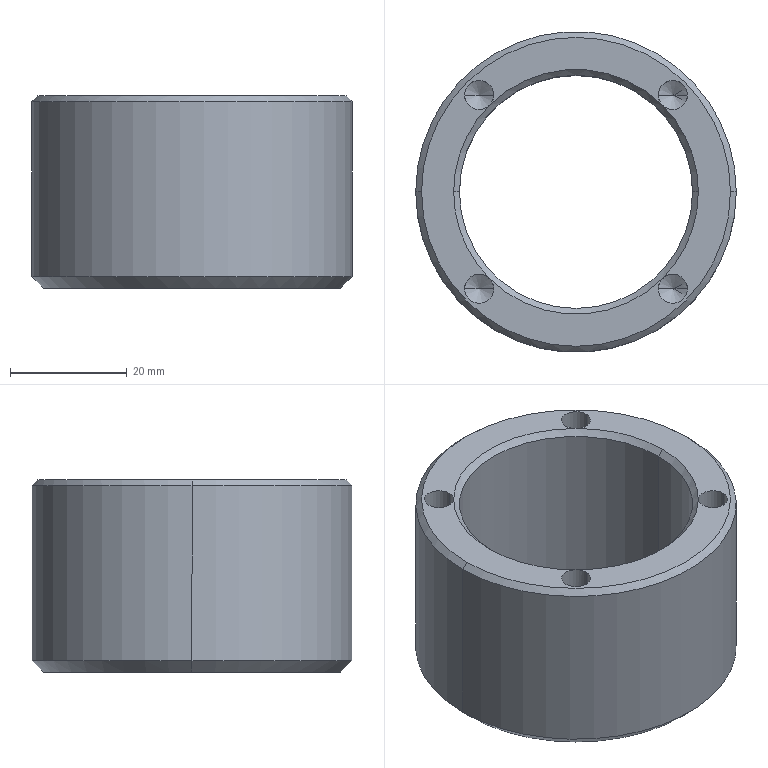Part | STEP file | Locating post-Mkt | 1 solid | 30 faces | box 55 x 55 x 33 mm | volume 35166 mm3 | cone 16 | cylinder 12 | plane 2 | commonest cylinder face diameters 5 x8 40 x2 55 x2